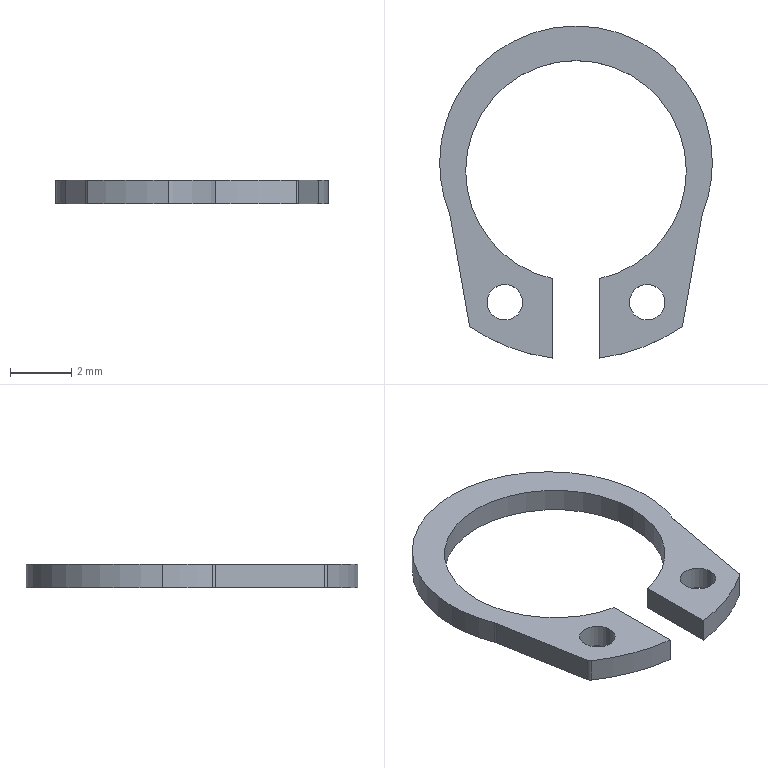Part | SolidWorks | features BaseBody 1 | 1 solid | 22 faces | box 8.901 x 10.834 x 0.774 mm | volume 24.698 mm3 | cylinder 16 | plane 6 | commonest cylinder face diameters 1.161 x4 7.198 x3 8.901 x3 0.31 x2 0.774 x2 12.307 x2
STEP:
#1=CARTESIAN_POINT('',(-2.903,-4.915,-0.387));
#2=VERTEX_POINT('',#1);
#3=CARTESIAN_POINT('',(-1.742,-4.915,-0.387));
#4=VERTEX_POINT('',#3);
#5=CARTESIAN_POINT('',(-2.322,-4.915,-0.387));
#6=DIRECTION('',(0.,0.,1.));
#7=DIRECTION('',(1.,0.,0.));
#8=AXIS2_PLACEMENT_3D('',#5,#6,#7);
#9=CIRCLE('',#8,0.5805);
#10=EDGE_CURVE('',#2,#4,#9,.T.);
#11=ORIENTED_EDGE('',*,*,#10,.T.);
#12=CARTESIAN_POINT('',(-2.322,-4.915,-0.387));
#13=DIRECTION('',(0.,0.,1.));
#14=DIRECTION('',(1.,0.,0.));
#15=AXIS2_PLACEMENT_3D('',#12,#13,#14);
#16=CIRCLE('',#15,0.5805);
#17=EDGE_CURVE('',#4,#2,#16,.T.);
#18=ORIENTED_EDGE('',*,*,#17,.T.);
#19=EDGE_LOOP('',(#11,#18));
#20=FACE_BOUND('',#19,.T.);
#21=CARTESIAN_POINT('',(1.742,-4.915,-0.387));
#22=VERTEX_POINT('',#21);
#23=CARTESIAN_POINT('',(2.903,-4.915,-0.387));
#24=VERTEX_POINT('',#23);
#25=CARTESIAN_POINT('',(2.322,-4.915,-0.387));
#26=DIRECTION('',(0.,0.,1.));
#27=DIRECTION('',(-1.,0.,0.));
#28=AXIS2_PLACEMENT_3D('',#25,#26,#27);
#29=CIRCLE('',#28,0.5805);
#30=EDGE_CURVE('',#22,#24,#29,.T.);
#31=ORIENTED_EDGE('',*,*,#30,.T.);
#32=CARTESIAN_POINT('',(2.322,-4.915,-0.387));
#33=DIRECTION('',(0.,0.,1.));
#34=DIRECTION('',(-1.,0.,0.));
#35=AXIS2_PLACEMENT_3D('',#32,#33,#34);
#36=CIRCLE('',#35,0.5805);
#37=EDGE_CURVE('',#24,#22,#36,.T.);
#38=ORIENTED_EDGE('',*,*,#37,.T.);
#39=EDGE_LOOP('',(#31,#38));
#40=FACE_BOUND('',#39,.T.);
#41=CARTESIAN_POINT('',(-4.134,-1.996,-0.387));
#42=VERTEX_POINT('',#41);
#43=CARTESIAN_POINT('',(-4.113,-2.072,-0.387));
#44=VERTEX_POINT('',#43);
#45=CARTESIAN_POINT('',(-4.494,-2.14,-0.387));
#46=DIRECTION('',(0.,0.,-1.));
#47=DIRECTION('',(1.,0.,0.));
#48=AXIS2_PLACEMENT_3D('',#45,#46,#47);
#49=CIRCLE('',#48,0.387);
#50=EDGE_CURVE('',#42,#44,#49,.T.);
#51=ORIENTED_EDGE('',*,*,#50,.F.);
#52=CARTESIAN_POINT('',(-4.45,-0.3485,-0.387));
#53=VERTEX_POINT('',#52);
#54=CARTESIAN_POINT('',(0.,-0.3485,-0.387));
#55=DIRECTION('',(0.,0.,1.));
#56=DIRECTION('',(1.,0.,0.));
#57=AXIS2_PLACEMENT_3D('',#54,#55,#56);
#58=CIRCLE('',#57,4.45);
#59=EDGE_CURVE('',#53,#42,#58,.T.);
#60=ORIENTED_EDGE('',*,*,#59,.F.);
#61=CARTESIAN_POINT('',(4.45,-0.3485,-0.387));
#62=VERTEX_POINT('',#61);
#63=CARTESIAN_POINT('',(0.,-0.3485,-0.387));
#64=DIRECTION('',(0.,0.,1.));
#65=DIRECTION('',(1.,0.,0.));
#66=AXIS2_PLACEMENT_3D('',#63,#64,#65);
#67=CIRCLE('',#66,4.45);
#68=EDGE_CURVE('',#62,#53,#67,.T.);
#69=ORIENTED_EDGE('',*,*,#68,.F.);
#70=CARTESIAN_POINT('',(4.134,-1.996,-0.387));
#71=VERTEX_POINT('',#70);
#72=CARTESIAN_POINT('',(0.,-0.3485,-0.387));
#73=DIRECTION('',(0.,0.,1.));
#74=DIRECTION('',(1.,0.,0.));
#75=AXIS2_PLACEMENT_3D('',#72,#73,#74);
#76=CIRCLE('',#75,4.45);
#77=EDGE_CURVE('',#71,#62,#76,.T.);
#78=ORIENTED_EDGE('',*,*,#77,.F.);
#79=CARTESIAN_POINT('',(4.113,-2.072,-0.387));
#80=VERTEX_POINT('',#79);
#81=CARTESIAN_POINT('',(4.494,-2.14,-0.387));
#82=DIRECTION('',(0.,0.,-1.));
#83=DIRECTION('',(-1.,0.,0.));
#84=AXIS2_PLACEMENT_3D('',#81,#82,#83);
#85=CIRCLE('',#84,0.387);
#86=EDGE_CURVE('',#80,#71,#85,.T.);
#87=ORIENTED_EDGE('',*,*,#86,.F.);
#88=CARTESIAN_POINT('',(3.483,-5.643,-0.387));
#89=VERTEX_POINT('',#88);
#90=CARTESIAN_POINT('',(4.113,-2.072,-0.387));
#91=DIRECTION('',(0.1736,0.9848,0.));
#92=VECTOR('',#91,1000.);
#93=LINE('',#90,#92);
#94=EDGE_CURVE('',#89,#80,#93,.T.);
#95=ORIENTED_EDGE('',*,*,#94,.F.);
#96=CARTESIAN_POINT('',(3.417,-5.745,-0.387));
#97=VERTEX_POINT('',#96);
#98=CARTESIAN_POINT('',(3.331,-5.616,-0.387));
#99=DIRECTION('',(0.,0.,1.));
#100=DIRECTION('',(1.,0.,0.));
#101=AXIS2_PLACEMENT_3D('',#98,#99,#100);
#102=CIRCLE('',#101,0.1548);
#103=EDGE_CURVE('',#97,#89,#102,.T.);
#104=ORIENTED_EDGE('',*,*,#103,.F.);
#105=CARTESIAN_POINT('',(0.774,-6.732,-0.387));
#106=VERTEX_POINT('',#105);
#107=CARTESIAN_POINT('',(0.,-0.6271,-0.387));
#108=DIRECTION('',(0.,0.,1.));
#109=DIRECTION('',(1.,0.,0.));
#110=AXIS2_PLACEMENT_3D('',#107,#108,#109);
#111=CIRCLE('',#110,6.153);
#112=EDGE_CURVE('',#106,#97,#111,.T.);
#113=ORIENTED_EDGE('',*,*,#112,.F.);
#114=CARTESIAN_POINT('',(0.774,-4.142,-0.387));
#115=VERTEX_POINT('',#114);
#116=CARTESIAN_POINT('',(0.774,-4.142,-0.387));
#117=DIRECTION('',(0.,-1.,0.));
#118=VECTOR('',#117,1000.);
#119=LINE('',#116,#118);
#120=EDGE_CURVE('',#115,#106,#119,.T.);
#121=ORIENTED_EDGE('',*,*,#120,.F.);
#122=CARTESIAN_POINT('',(3.599,-0.6271,-0.387));
#123=VERTEX_POINT('',#122);
#124=CARTESIAN_POINT('',(0.,-0.6271,-0.387));
#125=DIRECTION('',(0.,0.,-1.));
#126=DIRECTION('',(1.,0.,0.));
#127=AXIS2_PLACEMENT_3D('',#124,#125,#126);
#128=CIRCLE('',#127,3.599);
#129=EDGE_CURVE('',#123,#115,#128,.T.);
#130=ORIENTED_EDGE('',*,*,#129,.F.);
#131=CARTESIAN_POINT('',(-3.599,-0.6271,-0.387));
#132=VERTEX_POINT('',#131);
#133=CARTESIAN_POINT('',(0.,-0.6271,-0.387));
#134=DIRECTION('',(0.,0.,-1.));
#135=DIRECTION('',(1.,0.,0.));
#136=AXIS2_PLACEMENT_3D('',#133,#134,#135);
#137=CIRCLE('',#136,3.599);
#138=EDGE_CURVE('',#132,#123,#137,.T.);
#139=ORIENTED_EDGE('',*,*,#138,.F.);
#140=CARTESIAN_POINT('',(-0.774,-4.142,-0.387));
#141=VERTEX_POINT('',#140);
#142=CARTESIAN_POINT('',(0.,-0.6271,-0.387));
#143=DIRECTION('',(0.,0.,-1.));
#144=DIRECTION('',(1.,0.,0.));
#145=AXIS2_PLACEMENT_3D('',#142,#143,#144);
#146=CIRCLE('',#145,3.599);
#147=EDGE_CURVE('',#141,#132,#146,.T.);
#148=ORIENTED_EDGE('',*,*,#147,.F.);
#149=CARTESIAN_POINT('',(-0.774,-6.732,-0.387));
#150=VERTEX_POINT('',#149);
#151=CARTESIAN_POINT('',(-0.774,-4.142,-0.387));
#152=DIRECTION('',(0.,1.,0.));
#153=VECTOR('',#152,1000.);
#154=LINE('',#151,#153);
#155=EDGE_CURVE('',#150,#141,#154,.T.);
#156=ORIENTED_EDGE('',*,*,#155,.F.);
#157=CARTESIAN_POINT('',(-3.417,-5.745,-0.387));
#158=VERTEX_POINT('',#157);
#159=CARTESIAN_POINT('',(0.,-0.6271,-0.387));
#160=DIRECTION('',(0.,0.,1.));
#161=DIRECTION('',(-1.,0.,0.));
#162=AXIS2_PLACEMENT_3D('',#159,#160,#161);
#163=CIRCLE('',#162,6.153);
#164=EDGE_CURVE('',#158,#150,#163,.T.);
#165=ORIENTED_EDGE('',*,*,#164,.F.);
#166=CARTESIAN_POINT('',(-3.483,-5.643,-0.387));
#167=VERTEX_POINT('',#166);
#168=CARTESIAN_POINT('',(-3.331,-5.616,-0.387));
#169=DIRECTION('',(0.,0.,1.));
#170=DIRECTION('',(-1.,0.,0.));
#171=AXIS2_PLACEMENT_3D('',#168,#169,#170);
#172=CIRCLE('',#171,0.1548);
#173=EDGE_CURVE('',#167,#158,#172,.T.);
#174=ORIENTED_EDGE('',*,*,#173,.F.);
#175=CARTESIAN_POINT('',(-4.113,-2.072,-0.387));
#176=DIRECTION('',(0.1736,-0.9848,0.));
#177=VECTOR('',#176,1000.);
#178=LINE('',#175,#177);
#179=EDGE_CURVE('',#44,#167,#178,.T.);
#180=ORIENTED_EDGE('',*,*,#179,.F.);
#181=EDGE_LOOP('',(#51,#60,#69,#78,#87,#95,#104,#113,#121,#130,#139,#148,#156,#165,#174,#180));
#182=FACE_OUTER_BOUND('',#181,.T.);
#183=CARTESIAN_POINT('',(-4.494,-2.14,-0.387));
#184=DIRECTION('',(0.,0.,1.));
#185=DIRECTION('',(1.,0.,0.));
#186=AXIS2_PLACEMENT_3D('',#183,#184,#185);
#187=PLANE('',#186);
#188=ADVANCED_FACE('',(#20,#40,#182),#187,.F.);
#189=CARTESIAN_POINT('',(2.903,-4.915,0.387));
#190=VERTEX_POINT('',#189);
#191=CARTESIAN_POINT('',(2.903,-4.915,0.387));
#192=DIRECTION('',(0.,0.,-1.));
#193=VECTOR('',#192,1000.);
#194=LINE('',#191,#193);
#195=EDGE_CURVE('',#190,#24,#194,.T.);
#196=ORIENTED_EDGE('',*,*,#195,.F.);
#197=CARTESIAN_POINT('',(1.742,-4.915,0.387));
#198=VERTEX_POINT('',#197);
#199=CARTESIAN_POINT('',(2.322,-4.915,0.387));
#200=DIRECTION('',(0.,0.,1.));
#201=DIRECTION('',(-1.,0.,0.));
#202=AXIS2_PLACEMENT_3D('',#199,#200,#201);
#203=CIRCLE('',#202,0.5805);
#204=EDGE_CURVE('',#190,#198,#203,.T.);
#205=ORIENTED_EDGE('',*,*,#204,.T.);
#206=CARTESIAN_POINT('',(1.742,-4.915,0.387));
#207=DIRECTION('',(0.,0.,-1.));
#208=VECTOR('',#207,1000.);
#209=LINE('',#206,#208);
#210=EDGE_CURVE('',#198,#22,#209,.T.);
#211=ORIENTED_EDGE('',*,*,#210,.T.);
#212=ORIENTED_EDGE('',*,*,#37,.F.);
#213=EDGE_LOOP('',(#196,#205,#211,#212));
#214=FACE_OUTER_BOUND('',#213,.T.);
#215=CARTESIAN_POINT('',(2.322,-4.915,0.387));
#216=DIRECTION('',(0.,0.,-1.));
#217=DIRECTION('',(-1.,0.,0.));
#218=AXIS2_PLACEMENT_3D('',#215,#216,#217);
#219=CYLINDRICAL_SURFACE('',#218,0.5805);
#220=ADVANCED_FACE('',(#214),#219,.F.);
#221=CARTESIAN_POINT('',(-1.742,-4.915,0.387));
#222=VERTEX_POINT('',#221);
#223=CARTESIAN_POINT('',(-1.742,-4.915,0.387));
#224=DIRECTION('',(0.,0.,-1.));
#225=VECTOR('',#224,1000.);
#226=LINE('',#223,#225);
#227=EDGE_CURVE('',#222,#4,#226,.T.);
#228=ORIENTED_EDGE('',*,*,#227,.F.);
#229=CARTESIAN_POINT('',(-2.903,-4.915,0.387));
#230=VERTEX_POINT('',#229);
#231=CARTESIAN_POINT('',(-2.322,-4.915,0.387));
#232=DIRECTION('',(0.,0.,1.));
#233=DIRECTION('',(1.,0.,0.));
#234=AXIS2_PLACEMENT_3D('',#231,#232,#233);
#235=CIRCLE('',#234,0.5805);
#236=EDGE_CURVE('',#222,#230,#235,.T.);
#237=ORIENTED_EDGE('',*,*,#236,.T.);
#238=CARTESIAN_POINT('',(-2.903,-4.915,0.387));
#239=DIRECTION('',(0.,0.,-1.));
#240=VECTOR('',#239,1000.);
#241=LINE('',#238,#240);
#242=EDGE_CURVE('',#230,#2,#241,.T.);
#243=ORIENTED_EDGE('',*,*,#242,.T.);
#244=ORIENTED_EDGE('',*,*,#17,.F.);
#245=EDGE_LOOP('',(#228,#237,#243,#244));
#246=FACE_OUTER_BOUND('',#245,.T.);
#247=CARTESIAN_POINT('',(-2.322,-4.915,0.387));
#248=DIRECTION('',(0.,0.,-1.));
#249=DIRECTION('',(-1.,0.,0.));
#250=AXIS2_PLACEMENT_3D('',#247,#248,#249);
#251=CYLINDRICAL_SURFACE('',#250,0.5805);
#252=ADVANCED_FACE('',(#246),#251,.F.);
#253=CARTESIAN_POINT('',(4.45,-0.3485,0.387));
#254=VERTEX_POINT('',#253);
#255=CARTESIAN_POINT('',(4.45,-0.3485,0.387));
#256=DIRECTION('',(0.,0.,-1.));
#257=VECTOR('',#256,1000.);
#258=LINE('',#255,#257);
#259=EDGE_CURVE('',#254,#62,#258,.T.);
#260=ORIENTED_EDGE('',*,*,#259,.F.);
#261=CARTESIAN_POINT('',(4.134,-1.996,0.387));
#262=VERTEX_POINT('',#261);
#263=CARTESIAN_POINT('',(0.,-0.3485,0.387));
#264=DIRECTION('',(0.,0.,1.));
#265=DIRECTION('',(1.,0.,0.));
#266=AXIS2_PLACEMENT_3D('',#263,#264,#265);
#267=CIRCLE('',#266,4.45);
#268=EDGE_CURVE('',#262,#254,#267,.T.);
#269=ORIENTED_EDGE('',*,*,#268,.F.);
#270=CARTESIAN_POINT('',(4.134,-1.996,0.387));
#271=DIRECTION('',(0.,0.,-1.));
#272=VECTOR('',#271,1000.);
#273=LINE('',#270,#272);
#274=EDGE_CURVE('',#262,#71,#273,.T.);
#275=ORIENTED_EDGE('',*,*,#274,.T.);
#276=ORIENTED_EDGE('',*,*,#77,.T.);
#277=EDGE_LOOP('',(#260,#269,#275,#276));
#278=FACE_OUTER_BOUND('',#277,.T.);
#279=CARTESIAN_POINT('',(0.,-0.3485,0.387));
#280=DIRECTION('',(0.,0.,-1.));
#281=DIRECTION('',(-1.,0.,0.));
#282=AXIS2_PLACEMENT_3D('',#279,#280,#281);
#283=CYLINDRICAL_SURFACE('',#282,4.45);
#284=ADVANCED_FACE('',(#278),#283,.T.);
#285=CARTESIAN_POINT('',(4.113,-2.072,0.387));
#286=VERTEX_POINT('',#285);
#287=CARTESIAN_POINT('',(4.113,-2.072,0.387));
#288=DIRECTION('',(0.,0.,-1.));
#289=VECTOR('',#288,1000.);
#290=LINE('',#287,#289);
#291=EDGE_CURVE('',#286,#80,#290,.T.);
#292=ORIENTED_EDGE('',*,*,#291,.T.);
#293=ORIENTED_EDGE('',*,*,#86,.T.);
#294=ORIENTED_EDGE('',*,*,#274,.F.);
#295=CARTESIAN_POINT('',(4.494,-2.14,0.387));
#296=DIRECTION('',(0.,0.,-1.));
#297=DIRECTION('',(-1.,0.,0.));
#298=AXIS2_PLACEMENT_3D('',#295,#296,#297);
#299=CIRCLE('',#298,0.387);
#300=EDGE_CURVE('',#286,#262,#299,.T.);
#301=ORIENTED_EDGE('',*,*,#300,.F.);
#302=EDGE_LOOP('',(#292,#293,#294,#301));
#303=FACE_OUTER_BOUND('',#302,.T.);
#304=CARTESIAN_POINT('',(4.494,-2.14,0.387));
#305=DIRECTION('',(0.,0.,-1.));
#306=DIRECTION('',(-1.,0.,0.));
#307=AXIS2_PLACEMENT_3D('',#304,#305,#306);
#308=CYLINDRICAL_SURFACE('',#307,0.387);
#309=ADVANCED_FACE('',(#303),#308,.F.);
#310=CARTESIAN_POINT('',(3.483,-5.643,0.387));
#311=VERTEX_POINT('',#310);
#312=CARTESIAN_POINT('',(3.483,-5.643,0.387));
#313=DIRECTION('',(0.,0.,-1.));
#314=VECTOR('',#313,1000.);
#315=LINE('',#312,#314);
#316=EDGE_CURVE('',#311,#89,#315,.T.);
#317=ORIENTED_EDGE('',*,*,#316,.T.);
#318=ORIENTED_EDGE('',*,*,#94,.T.);
#319=ORIENTED_EDGE('',*,*,#291,.F.);
#320=CARTESIAN_POINT('',(4.113,-2.072,0.387));
#321=DIRECTION('',(0.1736,0.9848,0.));
#322=VECTOR('',#321,1000.);
#323=LINE('',#320,#322);
#324=EDGE_CURVE('',#311,#286,#323,.T.);
#325=ORIENTED_EDGE('',*,*,#324,.F.);
#326=EDGE_LOOP('',(#317,#318,#319,#325));
#327=FACE_OUTER_BOUND('',#326,.T.);
#328=CARTESIAN_POINT('',(4.113,-2.072,0.387));
#329=DIRECTION('',(-0.9848,0.1736,0.));
#330=DIRECTION('',(0.,0.,1.));
#331=AXIS2_PLACEMENT_3D('',#328,#329,#330);
#332=PLANE('',#331);
#333=ADVANCED_FACE('',(#327),#332,.F.);
#334=CARTESIAN_POINT('',(3.417,-5.745,0.387));
#335=VERTEX_POINT('',#334);
#336=CARTESIAN_POINT('',(3.417,-5.745,0.387));
#337=DIRECTION('',(0.,0.,-1.));
#338=VECTOR('',#337,1000.);
#339=LINE('',#336,#338);
#340=EDGE_CURVE('',#335,#97,#339,.T.);
#341=ORIENTED_EDGE('',*,*,#340,.T.);
#342=ORIENTED_EDGE('',*,*,#103,.T.);
#343=ORIENTED_EDGE('',*,*,#316,.F.);
#344=CARTESIAN_POINT('',(3.331,-5.616,0.387));
#345=DIRECTION('',(0.,0.,1.));
#346=DIRECTION('',(1.,0.,0.));
#347=AXIS2_PLACEMENT_3D('',#344,#345,#346);
#348=CIRCLE('',#347,0.1548);
#349=EDGE_CURVE('',#335,#311,#348,.T.);
#350=ORIENTED_EDGE('',*,*,#349,.F.);
#351=EDGE_LOOP('',(#341,#342,#343,#350));
#352=FACE_OUTER_BOUND('',#351,.T.);
#353=CARTESIAN_POINT('',(3.331,-5.616,0.387));
#354=DIRECTION('',(0.,0.,-1.));
#355=DIRECTION('',(-1.,0.,0.));
#356=AXIS2_PLACEMENT_3D('',#353,#354,#355);
#357=CYLINDRICAL_SURFACE('',#356,0.1548);
#358=ADVANCED_FACE('',(#352),#357,.T.);
#359=CARTESIAN_POINT('',(0.774,-6.732,0.387));
#360=VERTEX_POINT('',#359);
#361=CARTESIAN_POINT('',(0.774,-6.732,0.387));
#362=DIRECTION('',(0.,0.,-1.));
#363=VECTOR('',#362,1000.);
#364=LINE('',#361,#363);
#365=EDGE_CURVE('',#360,#106,#364,.T.);
#366=ORIENTED_EDGE('',*,*,#365,.T.);
#367=ORIENTED_EDGE('',*,*,#112,.T.);
#368=ORIENTED_EDGE('',*,*,#340,.F.);
#369=CARTESIAN_POINT('',(0.,-0.6271,0.387));
#370=DIRECTION('',(0.,0.,1.));
#371=DIRECTION('',(1.,0.,0.));
#372=AXIS2_PLACEMENT_3D('',#369,#370,#371);
#373=CIRCLE('',#372,6.153);
#374=EDGE_CURVE('',#360,#335,#373,.T.);
#375=ORIENTED_EDGE('',*,*,#374,.F.);
#376=EDGE_LOOP('',(#366,#367,#368,#375));
#377=FACE_OUTER_BOUND('',#376,.T.);
#378=CARTESIAN_POINT('',(0.,-0.6271,0.387));
#379=DIRECTION('',(0.,0.,-1.));
#380=DIRECTION('',(-1.,0.,0.));
#381=AXIS2_PLACEMENT_3D('',#378,#379,#380);
#382=CYLINDRICAL_SURFACE('',#381,6.153);
#383=ADVANCED_FACE('',(#377),#382,.T.);
#384=CARTESIAN_POINT('',(0.774,-4.142,0.387));
#385=VERTEX_POINT('',#384);
#386=CARTESIAN_POINT('',(0.774,-4.142,0.387));
#387=DIRECTION('',(0.,0.,-1.));
#388=VECTOR('',#387,1000.);
#389=LINE('',#386,#388);
#390=EDGE_CURVE('',#385,#115,#389,.T.);
#391=ORIENTED_EDGE('',*,*,#390,.T.);
#392=ORIENTED_EDGE('',*,*,#120,.T.);
#393=ORIENTED_EDGE('',*,*,#365,.F.);
#394=CARTESIAN_POINT('',(0.774,-4.142,0.387));
#395=DIRECTION('',(0.,-1.,0.));
#396=VECTOR('',#395,1000.);
#397=LINE('',#394,#396);
#398=EDGE_CURVE('',#385,#360,#397,.T.);
#399=ORIENTED_EDGE('',*,*,#398,.F.);
#400=EDGE_LOOP('',(#391,#392,#393,#399));
#401=FACE_OUTER_BOUND('',#400,.T.);
#402=CARTESIAN_POINT('',(0.774,-4.142,0.387));
#403=DIRECTION('',(1.,0.,0.));
#404=DIRECTION('',(0.,1.,0.));
#405=AXIS2_PLACEMENT_3D('',#402,#403,#404);
#406=PLANE('',#405);
#407=ADVANCED_FACE('',(#401),#406,.F.);
#408=CARTESIAN_POINT('',(-3.599,-0.6271,0.387));
#409=VERTEX_POINT('',#408);
#410=CARTESIAN_POINT('',(-3.599,-0.6271,0.387));
#411=DIRECTION('',(0.,0.,-1.));
#412=VECTOR('',#411,1000.);
#413=LINE('',#410,#412);
#414=EDGE_CURVE('',#409,#132,#413,.T.);
#415=ORIENTED_EDGE('',*,*,#414,.F.);
#416=CARTESIAN_POINT('',(-0.774,-4.142,0.387));
#417=VERTEX_POINT('',#416);
#418=CARTESIAN_POINT('',(0.,-0.6271,0.387));
#419=DIRECTION('',(0.,0.,-1.));
#420=DIRECTION('',(1.,0.,0.));
#421=AXIS2_PLACEMENT_3D('',#418,#419,#420);
#422=CIRCLE('',#421,3.599);
#423=EDGE_CURVE('',#417,#409,#422,.T.);
#424=ORIENTED_EDGE('',*,*,#423,.F.);
#425=CARTESIAN_POINT('',(-0.774,-4.142,0.387));
#426=DIRECTION('',(0.,0.,-1.));
#427=VECTOR('',#426,1000.);
#428=LINE('',#425,#427);
#429=EDGE_CURVE('',#417,#141,#428,.T.);
#430=ORIENTED_EDGE('',*,*,#429,.T.);
#431=ORIENTED_EDGE('',*,*,#147,.T.);
#432=EDGE_LOOP('',(#415,#424,#430,#431));
#433=FACE_OUTER_BOUND('',#432,.T.);
#434=CARTESIAN_POINT('',(0.,-0.6271,0.387));
#435=DIRECTION('',(0.,0.,-1.));
#436=DIRECTION('',(-1.,0.,0.));
#437=AXIS2_PLACEMENT_3D('',#434,#435,#436);
#438=CYLINDRICAL_SURFACE('',#437,3.599);
#439=ADVANCED_FACE('',(#433),#438,.F.);
#440=CARTESIAN_POINT('',(-0.774,-6.732,0.387));
#441=VERTEX_POINT('',#440);
#442=CARTESIAN_POINT('',(-0.774,-6.732,0.387));
#443=DIRECTION('',(0.,0.,-1.));
#444=VECTOR('',#443,1000.);
#445=LINE('',#442,#444);
#446=EDGE_CURVE('',#441,#150,#445,.T.);
#447=ORIENTED_EDGE('',*,*,#446,.T.);
#448=ORIENTED_EDGE('',*,*,#155,.T.);
#449=ORIENTED_EDGE('',*,*,#429,.F.);
#450=CARTESIAN_POINT('',(-0.774,-4.142,0.387));
#451=DIRECTION('',(0.,1.,0.));
#452=VECTOR('',#451,1000.);
#453=LINE('',#450,#452);
#454=EDGE_CURVE('',#441,#417,#453,.T.);
#455=ORIENTED_EDGE('',*,*,#454,.F.);
#456=EDGE_LOOP('',(#447,#448,#449,#455));
#457=FACE_OUTER_BOUND('',#456,.T.);
#458=CARTESIAN_POINT('',(-0.774,-4.142,0.387));
#459=DIRECTION('',(-1.,0.,0.));
#460=DIRECTION('',(0.,1.,0.));
#461=AXIS2_PLACEMENT_3D('',#458,#459,#460);
#462=PLANE('',#461);
#463=ADVANCED_FACE('',(#457),#462,.F.);
#464=CARTESIAN_POINT('',(-3.417,-5.745,0.387));
#465=VERTEX_POINT('',#464);
#466=CARTESIAN_POINT('',(-3.417,-5.745,0.387));
#467=DIRECTION('',(0.,0.,-1.));
#468=VECTOR('',#467,1000.);
#469=LINE('',#466,#468);
#470=EDGE_CURVE('',#465,#158,#469,.T.);
#471=ORIENTED_EDGE('',*,*,#470,.T.);
#472=ORIENTED_EDGE('',*,*,#164,.T.);
#473=ORIENTED_EDGE('',*,*,#446,.F.);
#474=CARTESIAN_POINT('',(0.,-0.6271,0.387));
#475=DIRECTION('',(0.,0.,1.));
#476=DIRECTION('',(-1.,0.,0.));
#477=AXIS2_PLACEMENT_3D('',#474,#475,#476);
#478=CIRCLE('',#477,6.153);
#479=EDGE_CURVE('',#465,#441,#478,.T.);
#480=ORIENTED_EDGE('',*,*,#479,.F.);
#481=EDGE_LOOP('',(#471,#472,#473,#480));
#482=FACE_OUTER_BOUND('',#481,.T.);
#483=CARTESIAN_POINT('',(0.,-0.6271,0.387));
#484=DIRECTION('',(0.,0.,-1.));
#485=DIRECTION('',(-1.,0.,0.));
#486=AXIS2_PLACEMENT_3D('',#483,#484,#485);
#487=CYLINDRICAL_SURFACE('',#486,6.153);
#488=ADVANCED_FACE('',(#482),#487,.T.);
#489=CARTESIAN_POINT('',(-3.483,-5.643,0.387));
#490=VERTEX_POINT('',#489);
#491=CARTESIAN_POINT('',(-3.483,-5.643,0.387));
#492=DIRECTION('',(0.,0.,-1.));
#493=VECTOR('',#492,1000.);
#494=LINE('',#491,#493);
#495=EDGE_CURVE('',#490,#167,#494,.T.);
#496=ORIENTED_EDGE('',*,*,#495,.T.);
#497=ORIENTED_EDGE('',*,*,#173,.T.);
#498=ORIENTED_EDGE('',*,*,#470,.F.);
#499=CARTESIAN_POINT('',(-3.331,-5.616,0.387));
#500=DIRECTION('',(0.,0.,1.));
#501=DIRECTION('',(-1.,0.,0.));
#502=AXIS2_PLACEMENT_3D('',#499,#500,#501);
#503=CIRCLE('',#502,0.1548);
#504=EDGE_CURVE('',#490,#465,#503,.T.);
#505=ORIENTED_EDGE('',*,*,#504,.F.);
#506=EDGE_LOOP('',(#496,#497,#498,#505));
#507=FACE_OUTER_BOUND('',#506,.T.);
#508=CARTESIAN_POINT('',(-3.331,-5.616,0.387));
#509=DIRECTION('',(0.,0.,-1.));
#510=DIRECTION('',(-1.,0.,0.));
#511=AXIS2_PLACEMENT_3D('',#508,#509,#510);
#512=CYLINDRICAL_SURFACE('',#511,0.1548);
#513=ADVANCED_FACE('',(#507),#512,.T.);
#514=CARTESIAN_POINT('',(-4.113,-2.072,0.387));
#515=VERTEX_POINT('',#514);
#516=CARTESIAN_POINT('',(-4.113,-2.072,0.387));
#517=DIRECTION('',(0.,0.,-1.));
#518=VECTOR('',#517,1000.);
#519=LINE('',#516,#518);
#520=EDGE_CURVE('',#515,#44,#519,.T.);
#521=ORIENTED_EDGE('',*,*,#520,.T.);
#522=ORIENTED_EDGE('',*,*,#179,.T.);
#523=ORIENTED_EDGE('',*,*,#495,.F.);
#524=CARTESIAN_POINT('',(-4.113,-2.072,0.387));
#525=DIRECTION('',(0.1736,-0.9848,0.));
#526=VECTOR('',#525,1000.);
#527=LINE('',#524,#526);
#528=EDGE_CURVE('',#515,#490,#527,.T.);
#529=ORIENTED_EDGE('',*,*,#528,.F.);
#530=EDGE_LOOP('',(#521,#522,#523,#529));
#531=FACE_OUTER_BOUND('',#530,.T.);
#532=CARTESIAN_POINT('',(-4.113,-2.072,0.387));
#533=DIRECTION('',(0.9848,0.1736,0.));
#534=DIRECTION('',(0.,0.,-1.));
#535=AXIS2_PLACEMENT_3D('',#532,#533,#534);
#536=PLANE('',#535);
#537=ADVANCED_FACE('',(#531),#536,.F.);
#538=CARTESIAN_POINT('',(-4.134,-1.996,0.387));
#539=VERTEX_POINT('',#538);
#540=CARTESIAN_POINT('',(-4.134,-1.996,0.387));
#541=DIRECTION('',(0.,0.,-1.));
#542=VECTOR('',#541,1000.);
#543=LINE('',#540,#542);
#544=EDGE_CURVE('',#539,#42,#543,.T.);
#545=ORIENTED_EDGE('',*,*,#544,.T.);
#546=ORIENTED_EDGE('',*,*,#50,.T.);
#547=ORIENTED_EDGE('',*,*,#520,.F.);
#548=CARTESIAN_POINT('',(-4.494,-2.14,0.387));
#549=DIRECTION('',(0.,0.,-1.));
#550=DIRECTION('',(1.,0.,0.));
#551=AXIS2_PLACEMENT_3D('',#548,#549,#550);
#552=CIRCLE('',#551,0.387);
#553=EDGE_CURVE('',#539,#515,#552,.T.);
#554=ORIENTED_EDGE('',*,*,#553,.F.);
#555=EDGE_LOOP('',(#545,#546,#547,#554));
#556=FACE_OUTER_BOUND('',#555,.T.);
#557=CARTESIAN_POINT('',(-4.494,-2.14,0.387));
#558=DIRECTION('',(0.,0.,-1.));
#559=DIRECTION('',(-1.,0.,0.));
#560=AXIS2_PLACEMENT_3D('',#557,#558,#559);
#561=CYLINDRICAL_SURFACE('',#560,0.387);
#562=ADVANCED_FACE('',(#556),#561,.F.);
#563=CARTESIAN_POINT('',(2.322,-4.915,0.387));
#564=DIRECTION('',(0.,0.,1.));
#565=DIRECTION('',(-1.,0.,0.));
#566=AXIS2_PLACEMENT_3D('',#563,#564,#565);
#567=CIRCLE('',#566,0.5805);
#568=EDGE_CURVE('',#198,#190,#567,.T.);
#569=ORIENTED_EDGE('',*,*,#568,.F.);
#570=ORIENTED_EDGE('',*,*,#204,.F.);
#571=EDGE_LOOP('',(#569,#570));
#572=FACE_BOUND('',#571,.T.);
#573=CARTESIAN_POINT('',(-2.322,-4.915,0.387));
#574=DIRECTION('',(0.,0.,1.));
#575=DIRECTION('',(1.,0.,0.));
#576=AXIS2_PLACEMENT_3D('',#573,#574,#575);
#577=CIRCLE('',#576,0.5805);
#578=EDGE_CURVE('',#230,#222,#577,.T.);
#579=ORIENTED_EDGE('',*,*,#578,.F.);
#580=ORIENTED_EDGE('',*,*,#236,.F.);
#581=EDGE_LOOP('',(#579,#580));
#582=FACE_BOUND('',#581,.T.);
#583=ORIENTED_EDGE('',*,*,#553,.T.);
#584=ORIENTED_EDGE('',*,*,#528,.T.);
#585=ORIENTED_EDGE('',*,*,#504,.T.);
#586=ORIENTED_EDGE('',*,*,#479,.T.);
#587=ORIENTED_EDGE('',*,*,#454,.T.);
#588=ORIENTED_EDGE('',*,*,#423,.T.);
#589=CARTESIAN_POINT('',(3.599,-0.6271,0.387));
#590=VERTEX_POINT('',#589);
#591=CARTESIAN_POINT('',(0.,-0.6271,0.387));
#592=DIRECTION('',(0.,0.,-1.));
#593=DIRECTION('',(1.,0.,0.));
#594=AXIS2_PLACEMENT_3D('',#591,#592,#593);
#595=CIRCLE('',#594,3.599);
#596=EDGE_CURVE('',#409,#590,#595,.T.);
#597=ORIENTED_EDGE('',*,*,#596,.T.);
#598=CARTESIAN_POINT('',(0.,-0.6271,0.387));
#599=DIRECTION('',(0.,0.,-1.));
#600=DIRECTION('',(1.,0.,0.));
#601=AXIS2_PLACEMENT_3D('',#598,#599,#600);
#602=CIRCLE('',#601,3.599);
#603=EDGE_CURVE('',#590,#385,#602,.T.);
#604=ORIENTED_EDGE('',*,*,#603,.T.);
#605=ORIENTED_EDGE('',*,*,#398,.T.);
#606=ORIENTED_EDGE('',*,*,#374,.T.);
#607=ORIENTED_EDGE('',*,*,#349,.T.);
#608=ORIENTED_EDGE('',*,*,#324,.T.);
#609=ORIENTED_EDGE('',*,*,#300,.T.);
#610=ORIENTED_EDGE('',*,*,#268,.T.);
#611=CARTESIAN_POINT('',(-4.45,-0.3485,0.387));
#612=VERTEX_POINT('',#611);
#613=CARTESIAN_POINT('',(0.,-0.3485,0.387));
#614=DIRECTION('',(0.,0.,1.));
#615=DIRECTION('',(1.,0.,0.));
#616=AXIS2_PLACEMENT_3D('',#613,#614,#615);
#617=CIRCLE('',#616,4.45);
#618=EDGE_CURVE('',#254,#612,#617,.T.);
#619=ORIENTED_EDGE('',*,*,#618,.T.);
#620=CARTESIAN_POINT('',(0.,-0.3485,0.387));
#621=DIRECTION('',(0.,0.,1.));
#622=DIRECTION('',(1.,0.,0.));
#623=AXIS2_PLACEMENT_3D('',#620,#621,#622);
#624=CIRCLE('',#623,4.45);
#625=EDGE_CURVE('',#612,#539,#624,.T.);
#626=ORIENTED_EDGE('',*,*,#625,.T.);
#627=EDGE_LOOP('',(#583,#584,#585,#586,#587,#588,#597,#604,#605,#606,#607,#608,#609,#610,#619,#626));
#628=FACE_OUTER_BOUND('',#627,.T.);
#629=CARTESIAN_POINT('',(-4.494,-2.14,0.387));
#630=DIRECTION('',(0.,0.,1.));
#631=DIRECTION('',(1.,0.,0.));
#632=AXIS2_PLACEMENT_3D('',#629,#630,#631);
#633=PLANE('',#632);
#634=ADVANCED_FACE('',(#572,#582,#628),#633,.T.);
#635=CARTESIAN_POINT('',(3.599,-0.6271,0.387));
#636=DIRECTION('',(0.,0.,-1.));
#637=VECTOR('',#636,1000.);
#638=LINE('',#635,#637);
#639=EDGE_CURVE('',#590,#123,#638,.T.);
#640=ORIENTED_EDGE('',*,*,#639,.F.);
#641=ORIENTED_EDGE('',*,*,#596,.F.);
#642=ORIENTED_EDGE('',*,*,#414,.T.);
#643=ORIENTED_EDGE('',*,*,#138,.T.);
#644=EDGE_LOOP('',(#640,#641,#642,#643));
#645=FACE_OUTER_BOUND('',#644,.T.);
#646=CARTESIAN_POINT('',(0.,-0.6271,0.387));
#647=DIRECTION('',(0.,0.,-1.));
#648=DIRECTION('',(-1.,0.,0.));
#649=AXIS2_PLACEMENT_3D('',#646,#647,#648);
#650=CYLINDRICAL_SURFACE('',#649,3.599);
#651=ADVANCED_FACE('',(#645),#650,.F.);
#652=ORIENTED_EDGE('',*,*,#603,.F.);
#653=ORIENTED_EDGE('',*,*,#639,.T.);
#654=ORIENTED_EDGE('',*,*,#129,.T.);
#655=ORIENTED_EDGE('',*,*,#390,.F.);
#656=EDGE_LOOP('',(#652,#653,#654,#655));
#657=FACE_OUTER_BOUND('',#656,.T.);
#658=CARTESIAN_POINT('',(0.,-0.6271,0.387));
#659=DIRECTION('',(0.,0.,-1.));
#660=DIRECTION('',(-1.,0.,0.));
#661=AXIS2_PLACEMENT_3D('',#658,#659,#660);
#662=CYLINDRICAL_SURFACE('',#661,3.599);
#663=ADVANCED_FACE('',(#657),#662,.F.);
#664=ORIENTED_EDGE('',*,*,#625,.F.);
#665=CARTESIAN_POINT('',(-4.45,-0.3485,0.387));
#666=DIRECTION('',(0.,0.,-1.));
#667=VECTOR('',#666,1000.);
#668=LINE('',#665,#667);
#669=EDGE_CURVE('',#612,#53,#668,.T.);
#670=ORIENTED_EDGE('',*,*,#669,.T.);
#671=ORIENTED_EDGE('',*,*,#59,.T.);
#672=ORIENTED_EDGE('',*,*,#544,.F.);
#673=EDGE_LOOP('',(#664,#670,#671,#672));
#674=FACE_OUTER_BOUND('',#673,.T.);
#675=CARTESIAN_POINT('',(0.,-0.3485,0.387));
#676=DIRECTION('',(0.,0.,-1.));
#677=DIRECTION('',(-1.,0.,0.));
#678=AXIS2_PLACEMENT_3D('',#675,#676,#677);
#679=CYLINDRICAL_SURFACE('',#678,4.45);
#680=ADVANCED_FACE('',(#674),#679,.T.);
#681=ORIENTED_EDGE('',*,*,#618,.F.);
#682=ORIENTED_EDGE('',*,*,#259,.T.);
#683=ORIENTED_EDGE('',*,*,#68,.T.);
#684=ORIENTED_EDGE('',*,*,#669,.F.);
#685=EDGE_LOOP('',(#681,#682,#683,#684));
#686=FACE_OUTER_BOUND('',#685,.T.);
#687=CARTESIAN_POINT('',(0.,-0.3485,0.387));
#688=DIRECTION('',(0.,0.,-1.));
#689=DIRECTION('',(-1.,0.,0.));
#690=AXIS2_PLACEMENT_3D('',#687,#688,#689);
#691=CYLINDRICAL_SURFACE('',#690,4.45);
#692=ADVANCED_FACE('',(#686),#691,.T.);
#693=ORIENTED_EDGE('',*,*,#578,.T.);
#694=ORIENTED_EDGE('',*,*,#227,.T.);
#695=ORIENTED_EDGE('',*,*,#10,.F.);
#696=ORIENTED_EDGE('',*,*,#242,.F.);
#697=EDGE_LOOP('',(#693,#694,#695,#696));
#698=FACE_OUTER_BOUND('',#697,.T.);
#699=CARTESIAN_POINT('',(-2.322,-4.915,0.387));
#700=DIRECTION('',(0.,0.,-1.));
#701=DIRECTION('',(-1.,0.,0.));
#702=AXIS2_PLACEMENT_3D('',#699,#700,#701);
#703=CYLINDRICAL_SURFACE('',#702,0.5805);
#704=ADVANCED_FACE('',(#698),#703,.F.);
#705=ORIENTED_EDGE('',*,*,#568,.T.);
#706=ORIENTED_EDGE('',*,*,#195,.T.);
#707=ORIENTED_EDGE('',*,*,#30,.F.);
#708=ORIENTED_EDGE('',*,*,#210,.F.);
#709=EDGE_LOOP('',(#705,#706,#707,#708));
#710=FACE_OUTER_BOUND('',#709,.T.);
#711=CARTESIAN_POINT('',(2.322,-4.915,0.387));
#712=DIRECTION('',(0.,0.,-1.));
#713=DIRECTION('',(-1.,0.,0.));
#714=AXIS2_PLACEMENT_3D('',#711,#712,#713);
#715=CYLINDRICAL_SURFACE('',#714,0.5805);
#716=ADVANCED_FACE('',(#710),#715,.F.);
#717=CLOSED_SHELL('',(#188,#220,#252,#284,#309,#333,#358,#383,#407,#439,#463,#488,#513,#537,#562,#634,#651,#663,#680,#692,#704,#716));
#718=MANIFOLD_SOLID_BREP('',#717);
#719=CARTESIAN_POINT('',(0.,0.,0.));
#720=DIRECTION('',(0.,0.,1.));
#721=DIRECTION('',(1.,0.,0.));
#722=AXIS2_PLACEMENT_3D('',#719,#720,#721);
#723=(LENGTH_UNIT()NAMED_UNIT(*)SI_UNIT(.MILLI.,.METRE.));
#724=UNCERTAINTY_MEASURE_WITH_UNIT(LENGTH_MEASURE(0.00001),#723,'','');
#725=(NAMED_UNIT(*)PLANE_ANGLE_UNIT()SI_UNIT($,.RADIAN.));
#726=(NAMED_UNIT(*)SI_UNIT($,.STERADIAN.)SOLID_ANGLE_UNIT());
#727=(GEOMETRIC_REPRESENTATION_CONTEXT(3)GLOBAL_UNCERTAINTY_ASSIGNED_CONTEXT((#724))GLOBAL_UNIT_ASSIGNED_CONTEXT((#723,#725,#726))REPRESENTATION_CONTEXT('',''));
#728=ADVANCED_BREP_SHAPE_REPRESENTATION('',(#718,#722),#727);